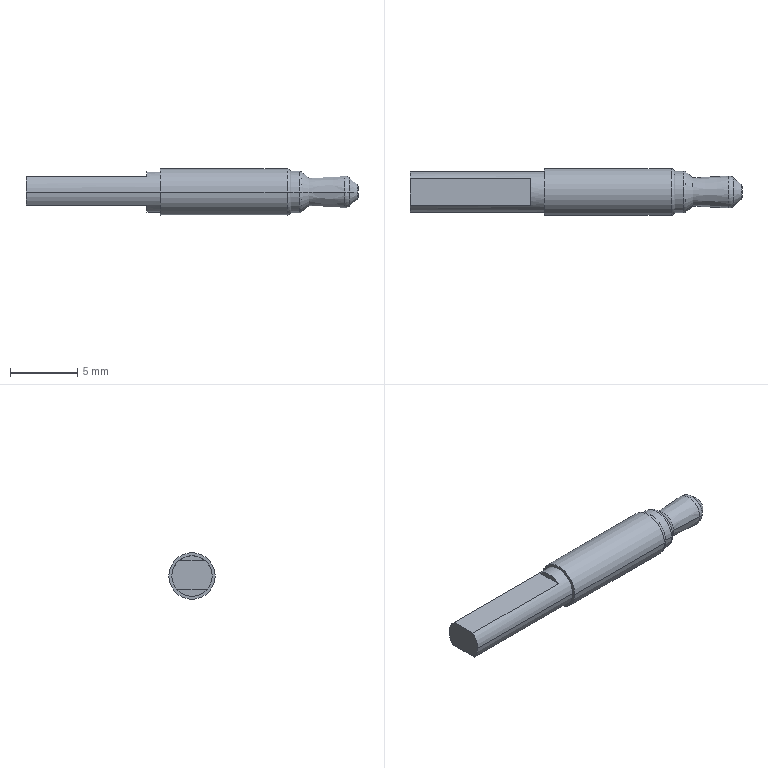Part | NX | 1 solid | 27 faces | box 24.7 x 3.45 x 3.45 mm | volume 171.24 mm3 | torus 8 | plane 7 | cylinder 6 | cone 6 | commonest cylinder face diameters 3 x2 3.1 x2 3.45 x2
STEP:
#1=CARTESIAN_POINT('',(12.641,-1.55,0.));
#2=VERTEX_POINT('',#1);
#3=CARTESIAN_POINT('',(12.641,1.55,0.));
#4=VERTEX_POINT('',#3);
#5=CARTESIAN_POINT('',(12.641,0.,0.));
#6=DIRECTION('',(1.,0.,0.));
#7=DIRECTION('',(0.,-1.,0.));
#8=AXIS2_PLACEMENT_3D('',#5,#6,#7);
#9=CIRCLE('',#8,1.55);
#10=EDGE_CURVE('',#2,#4,#9,.T.);
#11=ORIENTED_EDGE('',*,*,#10,.F.);
#12=CARTESIAN_POINT('',(12.,-1.55,0.));
#13=VERTEX_POINT('',#12);
#14=CARTESIAN_POINT('',(-0.85,-1.55,0.));
#15=DIRECTION('',(1.,0.,0.));
#16=VECTOR('',#15,1000.);
#17=LINE('',#14,#16);
#18=EDGE_CURVE('',#2,#13,#17,.F.);
#19=ORIENTED_EDGE('',*,*,#18,.T.);
#20=CARTESIAN_POINT('',(12.,1.55,0.));
#21=VERTEX_POINT('',#20);
#22=CARTESIAN_POINT('',(12.,0.,0.));
#23=DIRECTION('',(1.,0.,0.));
#24=DIRECTION('',(0.,1.,0.));
#25=AXIS2_PLACEMENT_3D('',#22,#23,#24);
#26=CIRCLE('',#25,1.55);
#27=EDGE_CURVE('',#13,#21,#26,.T.);
#28=ORIENTED_EDGE('',*,*,#27,.T.);
#29=CARTESIAN_POINT('',(-0.85,1.55,0.));
#30=DIRECTION('',(1.,0.,0.));
#31=VECTOR('',#30,1000.);
#32=LINE('',#29,#31);
#33=EDGE_CURVE('',#4,#21,#32,.F.);
#34=ORIENTED_EDGE('',*,*,#33,.F.);
#35=EDGE_LOOP('',(#11,#19,#28,#34));
#36=FACE_BOUND('',#35,.T.);
#37=CARTESIAN_POINT('',(-0.85,0.,0.));
#38=DIRECTION('',(1.,0.,0.));
#39=DIRECTION('',(0.,-1.,0.));
#40=AXIS2_PLACEMENT_3D('',#37,#38,#39);
#41=CYLINDRICAL_SURFACE('',#40,1.55);
#42=ADVANCED_FACE('',(#36),#41,.T.);
#43=CARTESIAN_POINT('',(13.35,-1.05,0.));
#44=VERTEX_POINT('',#43);
#45=CARTESIAN_POINT('',(13.35,1.05,0.));
#46=VERTEX_POINT('',#45);
#47=CARTESIAN_POINT('',(13.35,0.,0.));
#48=DIRECTION('',(1.,0.,0.));
#49=DIRECTION('',(0.,0.,-1.));
#50=AXIS2_PLACEMENT_3D('',#47,#48,#49);
#51=CIRCLE('',#50,1.05);
#52=EDGE_CURVE('',#44,#46,#51,.T.);
#53=ORIENTED_EDGE('',*,*,#52,.F.);
#54=CARTESIAN_POINT('',(12.833,-1.48,0.));
#55=VERTEX_POINT('',#54);
#56=CARTESIAN_POINT('',(13.05,-1.3,0.));
#57=DIRECTION('',(-0.7682,-0.6402,0.));
#58=VECTOR('',#57,1000.);
#59=LINE('',#56,#58);
#60=EDGE_CURVE('',#44,#55,#59,.T.);
#61=ORIENTED_EDGE('',*,*,#60,.T.);
#62=CARTESIAN_POINT('',(12.833,1.48,0.));
#63=VERTEX_POINT('',#62);
#64=CARTESIAN_POINT('',(12.833,0.,0.));
#65=DIRECTION('',(1.,0.,0.));
#66=DIRECTION('',(0.,-1.,0.));
#67=AXIS2_PLACEMENT_3D('',#64,#65,#66);
#68=CIRCLE('',#67,1.48);
#69=EDGE_CURVE('',#55,#63,#68,.T.);
#70=ORIENTED_EDGE('',*,*,#69,.T.);
#71=CARTESIAN_POINT('',(13.05,1.3,0.));
#72=DIRECTION('',(-0.7682,0.6402,0.));
#73=VECTOR('',#72,1000.);
#74=LINE('',#71,#73);
#75=EDGE_CURVE('',#46,#63,#74,.T.);
#76=ORIENTED_EDGE('',*,*,#75,.F.);
#77=EDGE_LOOP('',(#53,#61,#70,#76));
#78=FACE_BOUND('',#77,.T.);
#79=CARTESIAN_POINT('',(13.05,0.,0.));
#80=DIRECTION('',(-1.,0.,0.));
#81=DIRECTION('',(0.,1.,0.));
#82=AXIS2_PLACEMENT_3D('',#79,#80,#81);
#83=CONICAL_SURFACE('',#82,1.3,0.6947);
#84=ADVANCED_FACE('',(#78),#83,.T.);
#85=CARTESIAN_POINT('',(16.932,0.5598,0.));
#86=VERTEX_POINT('',#85);
#87=CARTESIAN_POINT('',(16.932,-0.5598,0.));
#88=VERTEX_POINT('',#87);
#89=CARTESIAN_POINT('',(16.932,0.,0.));
#90=DIRECTION('',(-1.,0.,0.));
#91=DIRECTION('',(0.,-1.,0.));
#92=AXIS2_PLACEMENT_3D('',#89,#90,#91);
#93=CIRCLE('',#92,0.5598);
#94=EDGE_CURVE('',#86,#88,#93,.T.);
#95=ORIENTED_EDGE('',*,*,#94,.T.);
#96=CARTESIAN_POINT('',(16.353,-1.066,0.));
#97=VERTEX_POINT('',#96);
#98=CARTESIAN_POINT('',(16.596,-0.8531,0.));
#99=DIRECTION('',(-0.7526,-0.6585,0.));
#100=VECTOR('',#99,1000.);
#101=LINE('',#98,#100);
#102=EDGE_CURVE('',#88,#97,#101,.T.);
#103=ORIENTED_EDGE('',*,*,#102,.T.);
#104=CARTESIAN_POINT('',(16.353,1.066,0.));
#105=VERTEX_POINT('',#104);
#106=CARTESIAN_POINT('',(16.353,0.,0.));
#107=DIRECTION('',(-1.,0.,0.));
#108=DIRECTION('',(0.,1.,0.));
#109=AXIS2_PLACEMENT_3D('',#106,#107,#108);
#110=CIRCLE('',#109,1.066);
#111=EDGE_CURVE('',#105,#97,#110,.T.);
#112=ORIENTED_EDGE('',*,*,#111,.F.);
#113=CARTESIAN_POINT('',(16.596,0.8531,0.));
#114=DIRECTION('',(-0.7526,0.6585,0.));
#115=VECTOR('',#114,1000.);
#116=LINE('',#113,#115);
#117=EDGE_CURVE('',#86,#105,#116,.T.);
#118=ORIENTED_EDGE('',*,*,#117,.F.);
#119=EDGE_LOOP('',(#95,#103,#112,#118));
#120=FACE_BOUND('',#119,.T.);
#121=CARTESIAN_POINT('',(16.596,0.,0.));
#122=DIRECTION('',(-1.,0.,0.));
#123=DIRECTION('',(0.,1.,0.));
#124=AXIS2_PLACEMENT_3D('',#121,#122,#123);
#125=CONICAL_SURFACE('',#124,0.8531,0.7188);
#126=ADVANCED_FACE('',(#120),#125,.T.);
#127=CARTESIAN_POINT('',(17.,-0.4092,0.));
#128=VERTEX_POINT('',#127);
#129=CARTESIAN_POINT('',(17.,0.4092,0.));
#130=VERTEX_POINT('',#129);
#131=CARTESIAN_POINT('',(17.,0.,0.));
#132=DIRECTION('',(-1.,0.,0.));
#133=DIRECTION('',(0.,1.,0.));
#134=AXIS2_PLACEMENT_3D('',#131,#132,#133);
#135=CIRCLE('',#134,0.4092);
#136=EDGE_CURVE('',#128,#130,#135,.T.);
#137=ORIENTED_EDGE('',*,*,#136,.F.);
#138=CARTESIAN_POINT('',(17.,0.,0.));
#139=DIRECTION('',(-1.,0.,0.));
#140=DIRECTION('',(0.,1.,0.));
#141=AXIS2_PLACEMENT_3D('',#138,#139,#140);
#142=CIRCLE('',#141,0.4092);
#143=EDGE_CURVE('',#130,#128,#142,.T.);
#144=ORIENTED_EDGE('',*,*,#143,.F.);
#145=EDGE_LOOP('',(#137,#144));
#146=FACE_BOUND('',#145,.T.);
#147=CARTESIAN_POINT('',(17.,0.,0.));
#148=DIRECTION('',(1.,0.,0.));
#149=DIRECTION('',(0.,1.,0.));
#150=AXIS2_PLACEMENT_3D('',#147,#148,#149);
#151=PLANE('',#150);
#152=ADVANCED_FACE('',(#146),#151,.T.);
#153=ORIENTED_EDGE('',*,*,#27,.F.);
#154=CARTESIAN_POINT('',(11.727,-1.725,0.));
#155=VERTEX_POINT('',#154);
#156=CARTESIAN_POINT('',(11.727,-1.425,0.));
#157=DIRECTION('',(0.,0.,-1.));
#158=DIRECTION('',(-1.,0.,0.));
#159=AXIS2_PLACEMENT_3D('',#156,#157,#158);
#160=CIRCLE('',#159,0.3);
#161=EDGE_CURVE('',#155,#13,#160,.F.);
#162=ORIENTED_EDGE('',*,*,#161,.F.);
#163=CARTESIAN_POINT('',(11.727,1.725,0.));
#164=VERTEX_POINT('',#163);
#165=CARTESIAN_POINT('',(11.727,0.,0.));
#166=DIRECTION('',(1.,0.,0.));
#167=DIRECTION('',(0.,-1.,0.));
#168=AXIS2_PLACEMENT_3D('',#165,#166,#167);
#169=CIRCLE('',#168,1.725);
#170=EDGE_CURVE('',#155,#164,#169,.T.);
#171=ORIENTED_EDGE('',*,*,#170,.T.);
#172=CARTESIAN_POINT('',(11.727,1.425,0.));
#173=DIRECTION('',(0.,0.,1.));
#174=DIRECTION('',(-1.,0.,0.));
#175=AXIS2_PLACEMENT_3D('',#172,#173,#174);
#176=CIRCLE('',#175,0.3);
#177=EDGE_CURVE('',#164,#21,#176,.F.);
#178=ORIENTED_EDGE('',*,*,#177,.T.);
#179=EDGE_LOOP('',(#153,#162,#171,#178));
#180=FACE_BOUND('',#179,.T.);
#181=CARTESIAN_POINT('',(11.727,0.,0.));
#182=DIRECTION('',(1.,0.,0.));
#183=DIRECTION('',(0.,-1.,0.));
#184=AXIS2_PLACEMENT_3D('',#181,#182,#183);
#185=TOROIDAL_SURFACE('',#184,1.425,0.3);
#186=ADVANCED_FACE('',(#180),#185,.T.);
#187=ORIENTED_EDGE('',*,*,#111,.T.);
#188=CARTESIAN_POINT('',(15.997,-1.189,0.));
#189=VERTEX_POINT('',#188);
#190=CARTESIAN_POINT('',(16.024,-0.69,0.));
#191=DIRECTION('',(0.,0.,1.));
#192=DIRECTION('',(-1.,0.,0.));
#193=AXIS2_PLACEMENT_3D('',#190,#191,#192);
#194=CIRCLE('',#193,0.5);
#195=EDGE_CURVE('',#189,#97,#194,.T.);
#196=ORIENTED_EDGE('',*,*,#195,.F.);
#197=CARTESIAN_POINT('',(15.997,1.189,0.));
#198=VERTEX_POINT('',#197);
#199=CARTESIAN_POINT('',(15.997,0.,0.));
#200=DIRECTION('',(-1.,0.,0.));
#201=DIRECTION('',(0.,1.,0.));
#202=AXIS2_PLACEMENT_3D('',#199,#200,#201);
#203=CIRCLE('',#202,1.189);
#204=EDGE_CURVE('',#198,#189,#203,.T.);
#205=ORIENTED_EDGE('',*,*,#204,.F.);
#206=CARTESIAN_POINT('',(16.024,0.69,0.));
#207=DIRECTION('',(0.,0.,-1.));
#208=DIRECTION('',(-1.,0.,0.));
#209=AXIS2_PLACEMENT_3D('',#206,#207,#208);
#210=CIRCLE('',#209,0.5);
#211=EDGE_CURVE('',#198,#105,#210,.T.);
#212=ORIENTED_EDGE('',*,*,#211,.T.);
#213=EDGE_LOOP('',(#187,#196,#205,#212));
#214=FACE_BOUND('',#213,.T.);
#215=CARTESIAN_POINT('',(16.024,0.,0.));
#216=DIRECTION('',(-1.,0.,0.));
#217=DIRECTION('',(0.,1.,0.));
#218=AXIS2_PLACEMENT_3D('',#215,#216,#217);
#219=TOROIDAL_SURFACE('',#218,0.69,0.5);
#220=ADVANCED_FACE('',(#214),#219,.T.);
#221=CARTESIAN_POINT('',(2.3,1.725,0.));
#222=VERTEX_POINT('',#221);
#223=CARTESIAN_POINT('',(2.3,-1.725,0.));
#224=VERTEX_POINT('',#223);
#225=CARTESIAN_POINT('',(2.3,0.,0.));
#226=DIRECTION('',(1.,0.,0.));
#227=DIRECTION('',(0.,-1.,0.));
#228=AXIS2_PLACEMENT_3D('',#225,#226,#227);
#229=CIRCLE('',#228,1.725);
#230=EDGE_CURVE('',#222,#224,#229,.T.);
#231=ORIENTED_EDGE('',*,*,#230,.T.);
#232=CARTESIAN_POINT('',(0.,-1.725,0.));
#233=DIRECTION('',(1.,0.,0.));
#234=VECTOR('',#233,1000.);
#235=LINE('',#232,#234);
#236=EDGE_CURVE('',#155,#224,#235,.F.);
#237=ORIENTED_EDGE('',*,*,#236,.F.);
#238=CARTESIAN_POINT('',(11.727,0.,0.));
#239=DIRECTION('',(1.,0.,0.));
#240=DIRECTION('',(0.,-1.,0.));
#241=AXIS2_PLACEMENT_3D('',#238,#239,#240);
#242=CIRCLE('',#241,1.725);
#243=EDGE_CURVE('',#164,#155,#242,.T.);
#244=ORIENTED_EDGE('',*,*,#243,.F.);
#245=CARTESIAN_POINT('',(0.,1.725,0.));
#246=DIRECTION('',(1.,0.,0.));
#247=VECTOR('',#246,1000.);
#248=LINE('',#245,#247);
#249=EDGE_CURVE('',#164,#222,#248,.F.);
#250=ORIENTED_EDGE('',*,*,#249,.T.);
#251=EDGE_LOOP('',(#231,#237,#244,#250));
#252=FACE_BOUND('',#251,.T.);
#253=CARTESIAN_POINT('',(0.,0.,0.));
#254=DIRECTION('',(1.,0.,0.));
#255=DIRECTION('',(0.,-1.,0.));
#256=AXIS2_PLACEMENT_3D('',#253,#254,#255);
#257=CYLINDRICAL_SURFACE('',#256,1.725);
#258=ADVANCED_FACE('',(#252),#257,.T.);
#259=ORIENTED_EDGE('',*,*,#204,.T.);
#260=CARTESIAN_POINT('',(14.734,-1.123,0.));
#261=DIRECTION('',(0.9986,-0.05256,0.));
#262=VECTOR('',#261,1000.);
#263=LINE('',#260,#262);
#264=EDGE_CURVE('',#189,#44,#263,.F.);
#265=ORIENTED_EDGE('',*,*,#264,.T.);
#266=ORIENTED_EDGE('',*,*,#52,.T.);
#267=CARTESIAN_POINT('',(14.734,1.123,0.));
#268=DIRECTION('',(0.9986,0.05256,0.));
#269=VECTOR('',#268,1000.);
#270=LINE('',#267,#269);
#271=EDGE_CURVE('',#198,#46,#270,.F.);
#272=ORIENTED_EDGE('',*,*,#271,.F.);
#273=EDGE_LOOP('',(#259,#265,#266,#272));
#274=FACE_BOUND('',#273,.T.);
#275=CARTESIAN_POINT('',(14.734,0.,0.));
#276=DIRECTION('',(1.,0.,0.));
#277=DIRECTION('',(0.,-1.,0.));
#278=AXIS2_PLACEMENT_3D('',#275,#276,#277);
#279=CONICAL_SURFACE('',#278,1.123,0.05258);
#280=ADVANCED_FACE('',(#274),#279,.T.);
#281=ORIENTED_EDGE('',*,*,#10,.T.);
#282=CARTESIAN_POINT('',(12.641,1.25,0.));
#283=DIRECTION('',(0.,0.,1.));
#284=DIRECTION('',(-1.,0.,0.));
#285=AXIS2_PLACEMENT_3D('',#282,#283,#284);
#286=CIRCLE('',#285,0.3);
#287=EDGE_CURVE('',#4,#63,#286,.F.);
#288=ORIENTED_EDGE('',*,*,#287,.T.);
#289=ORIENTED_EDGE('',*,*,#69,.F.);
#290=CARTESIAN_POINT('',(12.641,-1.25,0.));
#291=DIRECTION('',(0.,0.,-1.));
#292=DIRECTION('',(-1.,0.,0.));
#293=AXIS2_PLACEMENT_3D('',#290,#291,#292);
#294=CIRCLE('',#293,0.3);
#295=EDGE_CURVE('',#2,#55,#294,.F.);
#296=ORIENTED_EDGE('',*,*,#295,.F.);
#297=EDGE_LOOP('',(#281,#288,#289,#296));
#298=FACE_BOUND('',#297,.T.);
#299=CARTESIAN_POINT('',(12.641,0.,0.));
#300=DIRECTION('',(1.,0.,0.));
#301=DIRECTION('',(0.,-1.,0.));
#302=AXIS2_PLACEMENT_3D('',#299,#300,#301);
#303=TOROIDAL_SURFACE('',#302,1.25,0.3);
#304=ADVANCED_FACE('',(#298),#303,.T.);
#305=ORIENTED_EDGE('',*,*,#136,.T.);
#306=CARTESIAN_POINT('',(16.8,0.4092,0.));
#307=DIRECTION('',(0.,0.,1.));
#308=DIRECTION('',(-1.,0.,0.));
#309=AXIS2_PLACEMENT_3D('',#306,#307,#308);
#310=CIRCLE('',#309,0.2);
#311=EDGE_CURVE('',#130,#86,#310,.T.);
#312=ORIENTED_EDGE('',*,*,#311,.T.);
#313=CARTESIAN_POINT('',(16.932,0.,0.));
#314=DIRECTION('',(-1.,0.,0.));
#315=DIRECTION('',(0.,-1.,0.));
#316=AXIS2_PLACEMENT_3D('',#313,#314,#315);
#317=CIRCLE('',#316,0.5598);
#318=EDGE_CURVE('',#88,#86,#317,.T.);
#319=ORIENTED_EDGE('',*,*,#318,.F.);
#320=CARTESIAN_POINT('',(16.8,-0.4092,0.));
#321=DIRECTION('',(0.,0.,-1.));
#322=DIRECTION('',(-1.,0.,0.));
#323=AXIS2_PLACEMENT_3D('',#320,#321,#322);
#324=CIRCLE('',#323,0.2);
#325=EDGE_CURVE('',#128,#88,#324,.T.);
#326=ORIENTED_EDGE('',*,*,#325,.F.);
#327=EDGE_LOOP('',(#305,#312,#319,#326));
#328=FACE_BOUND('',#327,.T.);
#329=CARTESIAN_POINT('',(16.8,0.,0.));
#330=DIRECTION('',(1.,0.,0.));
#331=DIRECTION('',(0.,-1.,0.));
#332=AXIS2_PLACEMENT_3D('',#329,#330,#331);
#333=TOROIDAL_SURFACE('',#332,0.4092,0.2);
#334=ADVANCED_FACE('',(#328),#333,.T.);
#335=ORIENTED_EDGE('',*,*,#230,.F.);
#336=CARTESIAN_POINT('',(2.3,0.,0.));
#337=DIRECTION('',(1.,0.,0.));
#338=DIRECTION('',(0.,-1.,0.));
#339=AXIS2_PLACEMENT_3D('',#336,#337,#338);
#340=CIRCLE('',#339,1.725);
#341=EDGE_CURVE('',#224,#222,#340,.T.);
#342=ORIENTED_EDGE('',*,*,#341,.F.);
#343=EDGE_LOOP('',(#335,#342));
#344=FACE_BOUND('',#343,.T.);
#345=CARTESIAN_POINT('',(2.3,1.5,0.));
#346=VERTEX_POINT('',#345);
#347=CARTESIAN_POINT('',(2.3,-1.5,0.));
#348=VERTEX_POINT('',#347);
#349=CARTESIAN_POINT('',(2.3,0.,0.));
#350=DIRECTION('',(-1.,0.,0.));
#351=DIRECTION('',(0.,-1.,0.));
#352=AXIS2_PLACEMENT_3D('',#349,#350,#351);
#353=CIRCLE('',#352,1.5);
#354=EDGE_CURVE('',#346,#348,#353,.T.);
#355=ORIENTED_EDGE('',*,*,#354,.F.);
#356=CARTESIAN_POINT('',(2.3,0.,0.));
#357=DIRECTION('',(-1.,0.,0.));
#358=DIRECTION('',(0.,-1.,0.));
#359=AXIS2_PLACEMENT_3D('',#356,#357,#358);
#360=CIRCLE('',#359,1.5);
#361=EDGE_CURVE('',#348,#346,#360,.T.);
#362=ORIENTED_EDGE('',*,*,#361,.F.);
#363=EDGE_LOOP('',(#355,#362));
#364=FACE_BOUND('',#363,.T.);
#365=CARTESIAN_POINT('',(2.3,-28.452,3.6));
#366=DIRECTION('',(1.,0.,0.));
#367=DIRECTION('',(0.,0.,1.));
#368=AXIS2_PLACEMENT_3D('',#365,#366,#367);
#369=PLANE('',#368);
#370=ADVANCED_FACE('',(#344,#364),#369,.F.);
#371=CARTESIAN_POINT('',(-7.7,1.5,0.));
#372=VERTEX_POINT('',#371);
#373=CARTESIAN_POINT('',(-7.7,1.144,-0.97));
#374=VERTEX_POINT('',#373);
#375=CARTESIAN_POINT('',(-7.7,0.,0.));
#376=DIRECTION('',(-1.,0.,0.));
#377=DIRECTION('',(0.,-1.,0.));
#378=AXIS2_PLACEMENT_3D('',#375,#376,#377);
#379=CIRCLE('',#378,1.5);
#380=EDGE_CURVE('',#372,#374,#379,.T.);
#381=ORIENTED_EDGE('',*,*,#380,.F.);
#382=CARTESIAN_POINT('',(2.3,1.5,0.));
#383=DIRECTION('',(-1.,0.,0.));
#384=VECTOR('',#383,1000.);
#385=LINE('',#382,#384);
#386=EDGE_CURVE('',#372,#346,#385,.F.);
#387=ORIENTED_EDGE('',*,*,#386,.T.);
#388=ORIENTED_EDGE('',*,*,#354,.T.);
#389=CARTESIAN_POINT('',(-7.7,-1.5,0.));
#390=VERTEX_POINT('',#389);
#391=CARTESIAN_POINT('',(2.3,-1.5,0.));
#392=DIRECTION('',(-1.,0.,0.));
#393=VECTOR('',#392,1000.);
#394=LINE('',#391,#393);
#395=EDGE_CURVE('',#390,#348,#394,.F.);
#396=ORIENTED_EDGE('',*,*,#395,.F.);
#397=CARTESIAN_POINT('',(-7.7,-1.144,-0.97));
#398=VERTEX_POINT('',#397);
#399=CARTESIAN_POINT('',(-7.7,0.,0.));
#400=DIRECTION('',(-1.,0.,0.));
#401=DIRECTION('',(0.,-1.,0.));
#402=AXIS2_PLACEMENT_3D('',#399,#400,#401);
#403=CIRCLE('',#402,1.5);
#404=EDGE_CURVE('',#398,#390,#403,.T.);
#405=ORIENTED_EDGE('',*,*,#404,.F.);
#406=CARTESIAN_POINT('',(1.3,-1.144,-0.97));
#407=VERTEX_POINT('',#406);
#408=CARTESIAN_POINT('',(2.3,-1.144,-0.97));
#409=DIRECTION('',(-1.,0.,0.));
#410=VECTOR('',#409,1000.);
#411=LINE('',#408,#410);
#412=EDGE_CURVE('',#398,#407,#411,.F.);
#413=ORIENTED_EDGE('',*,*,#412,.T.);
#414=CARTESIAN_POINT('',(1.3,1.144,-0.97));
#415=VERTEX_POINT('',#414);
#416=CARTESIAN_POINT('',(1.3,0.,0.));
#417=DIRECTION('',(-1.,0.,0.));
#418=DIRECTION('',(0.,-1.,0.));
#419=AXIS2_PLACEMENT_3D('',#416,#417,#418);
#420=CIRCLE('',#419,1.5);
#421=EDGE_CURVE('',#415,#407,#420,.T.);
#422=ORIENTED_EDGE('',*,*,#421,.F.);
#423=CARTESIAN_POINT('',(2.3,1.144,-0.97));
#424=DIRECTION('',(-1.,0.,0.));
#425=VECTOR('',#424,1000.);
#426=LINE('',#423,#425);
#427=EDGE_CURVE('',#374,#415,#426,.F.);
#428=ORIENTED_EDGE('',*,*,#427,.F.);
#429=EDGE_LOOP('',(#381,#387,#388,#396,#405,#413,#422,#428));
#430=FACE_BOUND('',#429,.T.);
#431=CARTESIAN_POINT('',(2.3,0.,0.));
#432=DIRECTION('',(-1.,0.,0.));
#433=DIRECTION('',(0.,-1.,0.));
#434=AXIS2_PLACEMENT_3D('',#431,#432,#433);
#435=CYLINDRICAL_SURFACE('',#434,1.5);
#436=ADVANCED_FACE('',(#430),#435,.T.);
#437=ORIENTED_EDGE('',*,*,#380,.T.);
#438=CARTESIAN_POINT('',(-7.7,0.,-0.97));
#439=DIRECTION('',(0.,1.,0.));
#440=VECTOR('',#439,1000.);
#441=LINE('',#438,#440);
#442=EDGE_CURVE('',#398,#374,#441,.T.);
#443=ORIENTED_EDGE('',*,*,#442,.F.);
#444=ORIENTED_EDGE('',*,*,#404,.T.);
#445=CARTESIAN_POINT('',(-7.7,-0.9864,1.13));
#446=VERTEX_POINT('',#445);
#447=CARTESIAN_POINT('',(-7.7,0.,0.));
#448=DIRECTION('',(-1.,0.,0.));
#449=DIRECTION('',(0.,-1.,0.));
#450=AXIS2_PLACEMENT_3D('',#447,#448,#449);
#451=CIRCLE('',#450,1.5);
#452=EDGE_CURVE('',#390,#446,#451,.T.);
#453=ORIENTED_EDGE('',*,*,#452,.T.);
#454=CARTESIAN_POINT('',(-7.7,0.9864,1.13));
#455=VERTEX_POINT('',#454);
#456=CARTESIAN_POINT('',(-7.7,0.,1.13));
#457=DIRECTION('',(0.,-1.,0.));
#458=VECTOR('',#457,1000.);
#459=LINE('',#456,#458);
#460=EDGE_CURVE('',#455,#446,#459,.T.);
#461=ORIENTED_EDGE('',*,*,#460,.F.);
#462=CARTESIAN_POINT('',(-7.7,0.,0.));
#463=DIRECTION('',(-1.,0.,0.));
#464=DIRECTION('',(0.,-1.,0.));
#465=AXIS2_PLACEMENT_3D('',#462,#463,#464);
#466=CIRCLE('',#465,1.5);
#467=EDGE_CURVE('',#455,#372,#466,.T.);
#468=ORIENTED_EDGE('',*,*,#467,.T.);
#469=EDGE_LOOP('',(#437,#443,#444,#453,#461,#468));
#470=FACE_BOUND('',#469,.T.);
#471=CARTESIAN_POINT('',(-7.7,0.6142,-0.2899));
#472=DIRECTION('',(-1.,0.,0.));
#473=DIRECTION('',(0.,0.,1.));
#474=AXIS2_PLACEMENT_3D('',#471,#472,#473);
#475=PLANE('',#474);
#476=ADVANCED_FACE('',(#470),#475,.T.);
#477=ORIENTED_EDGE('',*,*,#421,.T.);
#478=CARTESIAN_POINT('',(1.3,-1.5,-0.97));
#479=DIRECTION('',(0.,1.,0.));
#480=VECTOR('',#479,1000.);
#481=LINE('',#478,#480);
#482=EDGE_CURVE('',#407,#415,#481,.T.);
#483=ORIENTED_EDGE('',*,*,#482,.T.);
#484=EDGE_LOOP('',(#477,#483));
#485=FACE_BOUND('',#484,.T.);
#486=CARTESIAN_POINT('',(1.3,1.5,-2.47));
#487=DIRECTION('',(1.,0.,0.));
#488=DIRECTION('',(0.,0.,1.));
#489=AXIS2_PLACEMENT_3D('',#486,#487,#488);
#490=PLANE('',#489);
#491=ADVANCED_FACE('',(#485),#490,.F.);
#492=ORIENTED_EDGE('',*,*,#412,.F.);
#493=ORIENTED_EDGE('',*,*,#442,.T.);
#494=ORIENTED_EDGE('',*,*,#427,.T.);
#495=ORIENTED_EDGE('',*,*,#482,.F.);
#496=EDGE_LOOP('',(#492,#493,#494,#495));
#497=FACE_BOUND('',#496,.T.);
#498=CARTESIAN_POINT('',(-3.393,-0.2163,-0.97));
#499=DIRECTION('',(0.,0.,-1.));
#500=DIRECTION('',(0.,-1.,0.));
#501=AXIS2_PLACEMENT_3D('',#498,#499,#500);
#502=PLANE('',#501);
#503=ADVANCED_FACE('',(#497),#502,.T.);
#504=CARTESIAN_POINT('',(1.3,-0.9864,1.13));
#505=VERTEX_POINT('',#504);
#506=CARTESIAN_POINT('',(1.3,0.9864,1.13));
#507=VERTEX_POINT('',#506);
#508=CARTESIAN_POINT('',(1.3,0.,0.));
#509=DIRECTION('',(-1.,0.,0.));
#510=DIRECTION('',(0.,-1.,0.));
#511=AXIS2_PLACEMENT_3D('',#508,#509,#510);
#512=CIRCLE('',#511,1.5);
#513=EDGE_CURVE('',#505,#507,#512,.T.);
#514=ORIENTED_EDGE('',*,*,#513,.T.);
#515=CARTESIAN_POINT('',(1.3,-5.456,1.13));
#516=DIRECTION('',(0.,1.,0.));
#517=VECTOR('',#516,1000.);
#518=LINE('',#515,#517);
#519=EDGE_CURVE('',#505,#507,#518,.T.);
#520=ORIENTED_EDGE('',*,*,#519,.F.);
#521=EDGE_LOOP('',(#514,#520));
#522=FACE_BOUND('',#521,.T.);
#523=CARTESIAN_POINT('',(1.3,-5.456,3.53));
#524=DIRECTION('',(1.,0.,0.));
#525=DIRECTION('',(0.,1.,0.));
#526=AXIS2_PLACEMENT_3D('',#523,#524,#525);
#527=PLANE('',#526);
#528=ADVANCED_FACE('',(#522),#527,.F.);
#529=CARTESIAN_POINT('',(2.3,0.9864,1.13));
#530=DIRECTION('',(-1.,0.,0.));
#531=VECTOR('',#530,1000.);
#532=LINE('',#529,#531);
#533=EDGE_CURVE('',#507,#455,#532,.T.);
#534=ORIENTED_EDGE('',*,*,#533,.T.);
#535=ORIENTED_EDGE('',*,*,#460,.T.);
#536=CARTESIAN_POINT('',(2.3,-0.9864,1.13));
#537=DIRECTION('',(-1.,0.,0.));
#538=VECTOR('',#537,1000.);
#539=LINE('',#536,#538);
#540=EDGE_CURVE('',#505,#446,#539,.T.);
#541=ORIENTED_EDGE('',*,*,#540,.F.);
#542=ORIENTED_EDGE('',*,*,#519,.T.);
#543=EDGE_LOOP('',(#534,#535,#541,#542));
#544=FACE_BOUND('',#543,.T.);
#545=CARTESIAN_POINT('',(-5.112,-0.01314,1.13));
#546=DIRECTION('',(0.,0.,1.));
#547=DIRECTION('',(1.,0.,0.));
#548=AXIS2_PLACEMENT_3D('',#545,#546,#547);
#549=PLANE('',#548);
#550=ADVANCED_FACE('',(#544),#549,.T.);
#551=ORIENTED_EDGE('',*,*,#264,.F.);
#552=CARTESIAN_POINT('',(15.997,0.,0.));
#553=DIRECTION('',(-1.,0.,0.));
#554=DIRECTION('',(0.,1.,0.));
#555=AXIS2_PLACEMENT_3D('',#552,#553,#554);
#556=CIRCLE('',#555,1.189);
#557=EDGE_CURVE('',#189,#198,#556,.T.);
#558=ORIENTED_EDGE('',*,*,#557,.T.);
#559=ORIENTED_EDGE('',*,*,#271,.T.);
#560=CARTESIAN_POINT('',(13.35,0.,0.));
#561=DIRECTION('',(1.,0.,0.));
#562=DIRECTION('',(0.,0.,-1.));
#563=AXIS2_PLACEMENT_3D('',#560,#561,#562);
#564=CIRCLE('',#563,1.05);
#565=EDGE_CURVE('',#46,#44,#564,.T.);
#566=ORIENTED_EDGE('',*,*,#565,.T.);
#567=EDGE_LOOP('',(#551,#558,#559,#566));
#568=FACE_BOUND('',#567,.T.);
#569=CARTESIAN_POINT('',(14.734,0.,0.));
#570=DIRECTION('',(1.,0.,0.));
#571=DIRECTION('',(0.,-1.,0.));
#572=AXIS2_PLACEMENT_3D('',#569,#570,#571);
#573=CONICAL_SURFACE('',#572,1.123,0.05258);
#574=ADVANCED_FACE('',(#568),#573,.T.);
#575=ORIENTED_EDGE('',*,*,#395,.T.);
#576=ORIENTED_EDGE('',*,*,#361,.T.);
#577=ORIENTED_EDGE('',*,*,#386,.F.);
#578=ORIENTED_EDGE('',*,*,#467,.F.);
#579=ORIENTED_EDGE('',*,*,#533,.F.);
#580=ORIENTED_EDGE('',*,*,#513,.F.);
#581=ORIENTED_EDGE('',*,*,#540,.T.);
#582=ORIENTED_EDGE('',*,*,#452,.F.);
#583=EDGE_LOOP('',(#575,#576,#577,#578,#579,#580,#581,#582));
#584=FACE_BOUND('',#583,.T.);
#585=CARTESIAN_POINT('',(2.3,0.,0.));
#586=DIRECTION('',(-1.,0.,0.));
#587=DIRECTION('',(0.,-1.,0.));
#588=AXIS2_PLACEMENT_3D('',#585,#586,#587);
#589=CYLINDRICAL_SURFACE('',#588,1.5);
#590=ADVANCED_FACE('',(#584),#589,.T.);
#591=ORIENTED_EDGE('',*,*,#236,.T.);
#592=ORIENTED_EDGE('',*,*,#341,.T.);
#593=ORIENTED_EDGE('',*,*,#249,.F.);
#594=ORIENTED_EDGE('',*,*,#170,.F.);
#595=EDGE_LOOP('',(#591,#592,#593,#594));
#596=FACE_BOUND('',#595,.T.);
#597=CARTESIAN_POINT('',(0.,0.,0.));
#598=DIRECTION('',(1.,0.,0.));
#599=DIRECTION('',(0.,-1.,0.));
#600=AXIS2_PLACEMENT_3D('',#597,#598,#599);
#601=CYLINDRICAL_SURFACE('',#600,1.725);
#602=ADVANCED_FACE('',(#596),#601,.T.);
#603=ORIENTED_EDGE('',*,*,#117,.T.);
#604=CARTESIAN_POINT('',(16.353,0.,0.));
#605=DIRECTION('',(-1.,0.,0.));
#606=DIRECTION('',(0.,1.,0.));
#607=AXIS2_PLACEMENT_3D('',#604,#605,#606);
#608=CIRCLE('',#607,1.066);
#609=EDGE_CURVE('',#97,#105,#608,.T.);
#610=ORIENTED_EDGE('',*,*,#609,.F.);
#611=ORIENTED_EDGE('',*,*,#102,.F.);
#612=ORIENTED_EDGE('',*,*,#318,.T.);
#613=EDGE_LOOP('',(#603,#610,#611,#612));
#614=FACE_BOUND('',#613,.T.);
#615=CARTESIAN_POINT('',(16.596,0.,0.));
#616=DIRECTION('',(-1.,0.,0.));
#617=DIRECTION('',(0.,1.,0.));
#618=AXIS2_PLACEMENT_3D('',#615,#616,#617);
#619=CONICAL_SURFACE('',#618,0.8531,0.7188);
#620=ADVANCED_FACE('',(#614),#619,.T.);
#621=ORIENTED_EDGE('',*,*,#75,.T.);
#622=CARTESIAN_POINT('',(12.833,0.,0.));
#623=DIRECTION('',(1.,0.,0.));
#624=DIRECTION('',(0.,-1.,0.));
#625=AXIS2_PLACEMENT_3D('',#622,#623,#624);
#626=CIRCLE('',#625,1.48);
#627=EDGE_CURVE('',#63,#55,#626,.T.);
#628=ORIENTED_EDGE('',*,*,#627,.T.);
#629=ORIENTED_EDGE('',*,*,#60,.F.);
#630=ORIENTED_EDGE('',*,*,#565,.F.);
#631=EDGE_LOOP('',(#621,#628,#629,#630));
#632=FACE_BOUND('',#631,.T.);
#633=CARTESIAN_POINT('',(13.05,0.,0.));
#634=DIRECTION('',(-1.,0.,0.));
#635=DIRECTION('',(0.,1.,0.));
#636=AXIS2_PLACEMENT_3D('',#633,#634,#635);
#637=CONICAL_SURFACE('',#636,1.3,0.6947);
#638=ADVANCED_FACE('',(#632),#637,.T.);
#639=ORIENTED_EDGE('',*,*,#18,.F.);
#640=CARTESIAN_POINT('',(12.641,0.,0.));
#641=DIRECTION('',(1.,0.,0.));
#642=DIRECTION('',(0.,-1.,0.));
#643=AXIS2_PLACEMENT_3D('',#640,#641,#642);
#644=CIRCLE('',#643,1.55);
#645=EDGE_CURVE('',#4,#2,#644,.T.);
#646=ORIENTED_EDGE('',*,*,#645,.F.);
#647=ORIENTED_EDGE('',*,*,#33,.T.);
#648=CARTESIAN_POINT('',(12.,0.,0.));
#649=DIRECTION('',(1.,0.,0.));
#650=DIRECTION('',(0.,1.,0.));
#651=AXIS2_PLACEMENT_3D('',#648,#649,#650);
#652=CIRCLE('',#651,1.55);
#653=EDGE_CURVE('',#21,#13,#652,.T.);
#654=ORIENTED_EDGE('',*,*,#653,.T.);
#655=EDGE_LOOP('',(#639,#646,#647,#654));
#656=FACE_BOUND('',#655,.T.);
#657=CARTESIAN_POINT('',(-0.85,0.,0.));
#658=DIRECTION('',(1.,0.,0.));
#659=DIRECTION('',(0.,-1.,0.));
#660=AXIS2_PLACEMENT_3D('',#657,#658,#659);
#661=CYLINDRICAL_SURFACE('',#660,1.55);
#662=ADVANCED_FACE('',(#656),#661,.T.);
#663=ORIENTED_EDGE('',*,*,#243,.T.);
#664=ORIENTED_EDGE('',*,*,#161,.T.);
#665=ORIENTED_EDGE('',*,*,#653,.F.);
#666=ORIENTED_EDGE('',*,*,#177,.F.);
#667=EDGE_LOOP('',(#663,#664,#665,#666));
#668=FACE_BOUND('',#667,.T.);
#669=CARTESIAN_POINT('',(11.727,0.,0.));
#670=DIRECTION('',(1.,0.,0.));
#671=DIRECTION('',(0.,-1.,0.));
#672=AXIS2_PLACEMENT_3D('',#669,#670,#671);
#673=TOROIDAL_SURFACE('',#672,1.425,0.3);
#674=ADVANCED_FACE('',(#668),#673,.T.);
#675=ORIENTED_EDGE('',*,*,#211,.F.);
#676=ORIENTED_EDGE('',*,*,#557,.F.);
#677=ORIENTED_EDGE('',*,*,#195,.T.);
#678=ORIENTED_EDGE('',*,*,#609,.T.);
#679=EDGE_LOOP('',(#675,#676,#677,#678));
#680=FACE_BOUND('',#679,.T.);
#681=CARTESIAN_POINT('',(16.024,0.,0.));
#682=DIRECTION('',(-1.,0.,0.));
#683=DIRECTION('',(0.,1.,0.));
#684=AXIS2_PLACEMENT_3D('',#681,#682,#683);
#685=TOROIDAL_SURFACE('',#684,0.69,0.5);
#686=ADVANCED_FACE('',(#680),#685,.T.);
#687=ORIENTED_EDGE('',*,*,#295,.T.);
#688=ORIENTED_EDGE('',*,*,#627,.F.);
#689=ORIENTED_EDGE('',*,*,#287,.F.);
#690=ORIENTED_EDGE('',*,*,#645,.T.);
#691=EDGE_LOOP('',(#687,#688,#689,#690));
#692=FACE_BOUND('',#691,.T.);
#693=CARTESIAN_POINT('',(12.641,0.,0.));
#694=DIRECTION('',(1.,0.,0.));
#695=DIRECTION('',(0.,-1.,0.));
#696=AXIS2_PLACEMENT_3D('',#693,#694,#695);
#697=TOROIDAL_SURFACE('',#696,1.25,0.3);
#698=ADVANCED_FACE('',(#692),#697,.T.);
#699=ORIENTED_EDGE('',*,*,#94,.F.);
#700=ORIENTED_EDGE('',*,*,#311,.F.);
#701=ORIENTED_EDGE('',*,*,#143,.T.);
#702=ORIENTED_EDGE('',*,*,#325,.T.);
#703=EDGE_LOOP('',(#699,#700,#701,#702));
#704=FACE_BOUND('',#703,.T.);
#705=CARTESIAN_POINT('',(16.8,0.,0.));
#706=DIRECTION('',(1.,0.,0.));
#707=DIRECTION('',(0.,-1.,0.));
#708=AXIS2_PLACEMENT_3D('',#705,#706,#707);
#709=TOROIDAL_SURFACE('',#708,0.4092,0.2);
#710=ADVANCED_FACE('',(#704),#709,.T.);
#711=CLOSED_SHELL('',(#42,#84,#126,#152,#186,#220,#258,#280,#304,#334,#370,#436,#476,#491,#503,#528,#550,#574,#590,#602,#620,#638,#662,#674,#686,#698,#710));
#712=MANIFOLD_SOLID_BREP('',#711);
#713=(LENGTH_UNIT()NAMED_UNIT(*)SI_UNIT(.MILLI.,.METRE.));
#714=UNCERTAINTY_MEASURE_WITH_UNIT(LENGTH_MEASURE(0.00001),#713,'','');
#715=(NAMED_UNIT(*)PLANE_ANGLE_UNIT()SI_UNIT($,.RADIAN.));
#716=(NAMED_UNIT(*)SI_UNIT($,.STERADIAN.)SOLID_ANGLE_UNIT());
#717=(GEOMETRIC_REPRESENTATION_CONTEXT(3)GLOBAL_UNCERTAINTY_ASSIGNED_CONTEXT((#714))GLOBAL_UNIT_ASSIGNED_CONTEXT((#713,#715,#716))REPRESENTATION_CONTEXT('',''));
#718=ADVANCED_BREP_SHAPE_REPRESENTATION('',(#712),#717);